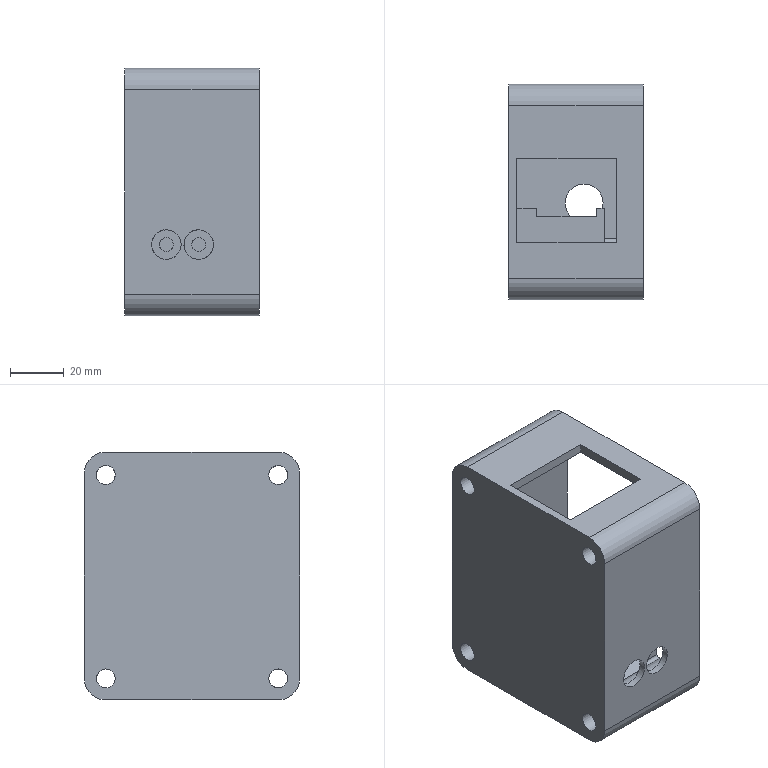NC program | NX | posted by the shop | part box 50 x 80 x 92 mm
Lines 170 to 1000 of 30419:
(T=6 N=D12-36-D12-120-3T-finish D=12.00 R=0.00 FL=45.00 L=120.00)
(XY-STOCK=0.15)
T6 M6
T7
G0 G90 G54 X-66.05 Y-33.361 S6500 M3
G43 H06 Z30.
M8
Z-22.
G1 X-65.9 Y-33.363 Z-22.937 F2000.
X-65.75 Y-33.364 Z-23.308
X-65.6 Y-33.365 Z-23.58
X-65.45 Y-33.367 Z-23.8
X-65.3 Y-33.368 Z-23.984
X-65.15 Y-33.369 Z-24.142
X-65. Y-33.371 Z-24.28
X-64.85 Y-33.372 Z-24.4
X-64.7 Y-33.374 Z-24.505
X-64.55 Y-33.375 Z-24.598
X-64.4 Y-33.376 Z-24.679
X-64.25 Y-33.378 Z-24.75
X-64.1 Y-33.379 Z-24.81
X-63.95 Y-33.38 Z-24.862
X-63.8 Y-33.382 Z-24.905
X-63.65 Y-33.383 Z-24.939
X-63.5 Y-33.384 Z-24.966
X-63.35 Y-33.386 Z-24.985
X-63.2 Y-33.387 Z-24.996
X-63.05 Y-33.388 Z-25.
X-61.193 Y-33.405
G3 X-60.033 Y-32.58 I.011 J1.212
X-59.585 Y-29.553 I-12.064 J3.334
X-59.432 Y-19.77 I-191.621 J7.885
G1 X-59.43 Y-16.803
Y47.501
G2 X-57.211 Y52.214 I6.58 J-.219
X-52.361 Y54.661 I7.101 J-8.045
X-46.379 Y55.335 I6.361 J-29.555
X-33.915 Y55.428 I9.594 J-450.446
G1 X51.556 Y55.427
G2 X56.253 Y53.174 I-.275 J-6.597
X58.654 Y48.401 I-8.065 J-7.048
X59.334 Y42.465 I-29.152 J-6.345
X59.43 Y29.326 I-461.878 J-9.943
G1 X59.428 Y-47.554
G2 X57.143 Y-52.281 I-6.607 J.278
X52.353 Y-54.664 I-7.048 J8.165
X46.506 Y-55.33 I-6.296 J29.24
X33.367 Y-55.428 I-9.91 J449.139
G1 X-51.541 Y-55.427
G2 X-56.242 Y-53.185 I.257 J6.591
X-58.663 Y-48.359 I8.09 J7.078
X-59.333 Y-42.467 I29.289 J6.315
X-59.39 Y-34.774 I126.794 J4.787
G3 X-58.934 Y-27.526 I-175.914 J14.706
X-58.831 Y-14.328 I-499.933 J10.525
G1 X-58.829 Y45.027
G2 X-55.109 Y51.907 I8.591 J-.199
X-49.637 Y54.134 I7.841 J-11.436
X-42.788 Y54.751 I7.155 J-41.068
X-30.144 Y54.828 I10.079 J-620.945
G1 X49.033 Y54.826
G2 X55.893 Y51.133 I-.197 J-8.582
X58.139 Y45.622 I-11.398 J-7.859
X58.754 Y38.728 I-41.439 J-7.174
X58.829 Y25.858 I-648.007 J-10.203
G1 X58.827 Y-45.032
G2 X55.145 Y-51.883 I-8.58 J.196
X49.633 Y-54.134 I-7.864 J11.38
X42.738 Y-54.753 I-7.179 J41.323
X29.869 Y-54.828 I-10.202 J645.306
G1 X-49.033 Y-54.826
G2 X-55.884 Y-51.143 I.197 J8.581
X-58.136 Y-45.633 I11.374 J7.863
X-58.75 Y-38.874 I40.722 J7.109
X-58.549 Y-31.841 I72.756 J1.438
G3 X-58.234 Y-17.292 I-249.929 J12.689
G1 X-58.231 Y-12.843
X-58.23 Y42.657
G2 X-55.478 Y49.812 I9.889 J.304
X-49.82 Y53.049 I8.956 J-9.091
X-43.473 Y54.025 I7.568 J-28.105
X-33.396 Y54.222 I8.68 J-185.849
G1 X-26.961 Y54.227
X46.784 Y54.226
G2 X55.547 Y49.295 I.185 J-9.925
X57.613 Y43.325 I-14.37 J-8.315
X58.167 Y35.836 I-53.023 J-7.684
X58.228 Y24.317 I-720.5 J-9.634
G1 X58.227 Y-42.782
G2 X53.365 Y-51.502 I-9.908 J-.191
X47.54 Y-53.574 I-8.277 J14.05
X40.415 Y-54.151 I-7.539 J48.744
X28.355 Y-54.227 I-10.043 J640.194
G1 X-46.784 Y-54.225
G2 X-55.479 Y-49.404 I-.194 J9.902
X-57.575 Y-43.538 I13.98 J8.304
X-58.04 Y-34.476 I43.348 J6.765
G3 X-57.633 Y-14.776 I-369.169 J17.479
G1 X-57.631 Y40.392
G2 X-57.018 Y45.008 I13.907 J.502
X-51.73 Y51.094 I10.34 J-3.644
X-45.529 Y53.036 I8.624 J-16.67
X-37.633 Y53.568 I8.096 J-61.247
X-25.258 Y53.627 I9.782 J-759.397
G1 X44.668 Y53.626
G2 X49.73 Y52.742 I.396 J-12.668
X55.242 Y47.456 I-4.495 J-10.203
X57.089 Y41.179 I-17.538 J-8.571
X57.584 Y32.829 I-69.072 J-8.283
X57.628 Y20.904 I-783.028 J-8.881
G1 X57.627 Y-40.667
G2 X56.744 Y-45.728 I-12.678 J-.395
X51.405 Y-51.266 I-10.214 J4.506
X45.121 Y-53.095 I-8.561 J17.702
X36.77 Y-53.583 I-8.272 J69.873
X24.89 Y-53.627 I-8.832 J782.468
G1 X-44.668 Y-53.626
G2 X-49.73 Y-52.742 I-.395 J12.678
X-55.267 Y-47.403 I4.505 J10.214
X-57.108 Y-40.985 I17.59 J8.517
X-57.351 Y-33.257 I49.862 J5.435
G3 X-57.032 Y-11.133 I-539.724 J18.847
G1 X-57.031 Y38.727
G2 X-56.496 Y43.45 I16.681 J.504
X-50.884 Y50.302 I11.023 J-3.304
X-44.446 Y52.375 I9.066 J-17.113
X-36.373 Y52.957 I8.421 J-60.577
X-23.999 Y53.026 I10.338 J-741.403
G1 X42.841 Y53.025
G2 X47.689 Y52.421 I.469 J-15.997
X54.309 Y46.873 I-3.551 J-10.961
X56.351 Y40.605 I-16.966 J-8.994
X56.956 Y32.489 I-58.8 J-8.463
X57.028 Y18.63 I-787.178 J-11.01
G1 X57.027 Y-38.822
G2 X56.454 Y-43.585 I-16.194 J-.469
X50.884 Y-50.301 I-10.979 J3.438
X44.563 Y-52.356 I-9.027 J17.015
X36.716 Y-52.949 I-8.324 J57.93
X23.847 Y-53.026 I-10.769 J722.444
G1 X-42.824 Y-53.025
G2 X-47.586 Y-52.453 I-.469 J16.195
X-54.302 Y-46.883 I3.438 J10.98
X-56.377 Y-40.245 I16.639 J8.843
X-56.692 Y-32.699 I49.548 J5.852
G3 X-56.432 Y-10.683 I-719.955 J19.513
G1 X-56.431 Y36.837
G2 X-56.043 Y41.626 I21.951 J.632
X-50.036 Y49.556 I11.703 J-2.625
X-43.439 Y51.721 I9.416 J-17.561
X-35.414 Y52.341 I8.614 J-59.257
X-20.925 Y52.426 I11.55 J-735.565
G1 X41.158 Y52.425
G2 X46.113 Y51.922 I.532 J-19.428
X53.596 Y45.967 I-3.122 J-11.602
X55.706 Y39.542 I-17.567 J-9.327
X56.338 Y31.608 I-57.664 J-8.586
X56.427 Y17.119 I-687.489 J-11.497
G1 Y-36.842
G2 X56.05 Y-41.587 I-22.034 J-.635
X49.974 Y-49.591 I-11.719 J2.589
X43.5 Y-51.71 I-9.349 J17.608
X35.251 Y-52.345 I-8.726 J59.472
X20.897 Y-52.426 I-11.543 J775.238
G1 X-40.843
G2 X-45.588 Y-52.048 I-.633 J22.054
X-53.592 Y-45.968 I2.578 J11.701
X-55.685 Y-39.254 I16.907 J8.953
X-56.036 Y-31.889 I51.489 J6.146
G3 X-55.833 Y-9.199 I-986.222 J20.177
G1 X-55.832 Y34.961
G2 X-55.538 Y39.941 I29.145 J.781
X-48.977 Y48.964 I12.341 J-2.077
X-42.365 Y51.093 I9.596 J-18.477
X-34.387 Y51.729 I8.768 J-59.601
X-19.358 Y51.826 I11.852 J-673.592
G1 X39.268 Y51.825
G2 X44.331 Y51.46 I.694 J-25.69
X52.873 Y45.143 I-2.432 J-12.222
X55.062 Y38.557 I-17.984 J-9.634
X55.726 Y30.536 I-57.633 J-8.813
X55.827 Y15.057 I-663.748 J-12.064
G1 Y-35.312
G2 X55.453 Y-40.374 I-25.27 J-.682
X49.038 Y-48.929 I-12.234 J2.491
X42.347 Y-51.095 I-9.65 J18.397
X33.873 Y-51.742 I-9.002 J62.053
X19.024 Y-51.826 I-11.863 J788.145
G1 X-39.313 Y-51.825
G2 X-44.376 Y-51.452 I-.682 J25.271
X-52.969 Y-44.944 I2.473 J12.194
X-55.022 Y-38.126 I17.756 J9.063
X-55.384 Y-30.265 I57.878 J6.605
G1 X-55.26 Y-19.515
X-55.233 Y-9.153
X-55.232 Y33.237
G2 X-54.977 Y38.536 I36.153 J.914
X-48.019 Y48.341 I12.855 J-1.75
X-41.178 Y50.494 I9.863 J-19.401
X-32.523 Y51.14 I9.224 J-65.201
X-17.673 Y51.225 I11.964 J-795.405
G1 X37.963 Y51.224
G2 X43.252 Y50.849 I.682 J-27.83
X52.246 Y44.194 I-2.418 J-12.674
X54.455 Y37.42 I-18.845 J-9.892
X55.137 Y28.723 I-62.607 J-9.285
X55.227 Y13.379 I-763.643 J-12.131
G1 X55.226 Y-33.962
G2 X54.85 Y-39.25 I-27.809 J-.682
X48.092 Y-48.3 I-12.7 J2.436
X41.165 Y-50.495 I-9.925 J19.292
X32.735 Y-51.135 I-9.114 J64.191
X17.391 Y-51.225 I-12.16 J764.582
G1 X-37.558
G2 X-42.809 Y-50.929 I-.816 J32.224
X-52.394 Y-43.858 I1.974 J12.708
X-54.374 Y-36.967 I18.877 J9.154
X-54.744 Y-28.611 I65.348 J7.079
G1 X-54.661 Y-19.337
X-54.633 Y-7.489
X-54.632 Y31.961
G2 X-54.367 Y37.485 I38.814 J.903
X-47.153 Y47.69 I13.26 J-1.722
X-40.185 Y49.872 I10.075 J-19.948
X-31.397 Y50.535 I9.43 J-66.433
X-16.052 Y50.625 I12.267 J-787.77
G1 X36.118 Y50.624
G2 X41.64 Y50.338 I.874 J-36.553
X51.695 Y43.143 I-1.864 J-13.227
X53.876 Y36.172 I-19.983 J-10.077
X54.531 Y27.563 I-65.673 J-9.328
X54.626 Y11.904 I-745.433 J-12.373
G1 Y-32.297
G2 X54.311 Y-37.817 I-34.27 J-.812
X47.178 Y-47.674 I-13.19 J2.035
X40.249 Y-49.861 I-10.075 J19.849
X31.686 Y-50.528 I-9.339 J64.607
X16.207 Y-50.625 I-12.277 J724.209
G1 X-36.298 Y-50.624
G2 X-41.818 Y-50.309 I-.812 J34.267
X-51.727 Y-42.979 I1.983 J13.043
X-53.712 Y-35.997 I19.559 J9.336
X-54.111 Y-27.552 I67.427 J7.418
G1 X-54.106 Y28.127
G2 X-53.946 Y34.695 I202.242 J-1.656
X-52.371 Y41.027 I16.21 J-.67
X-45.82 Y47.292 I12.448 J-6.458
X-38.708 Y49.333 I10.142 J-21.928
X-29.734 Y49.944 I9.569 J-74.278
X-14.884 Y50.024 I11.838 J-816.458
G1 X34.858
G2 X40.561 Y49.739 I.88 J-39.624
X51.063 Y42.273 I-1.773 J-13.612
X53.235 Y35.338 I-20.43 J-10.209
X53.915 Y26.821 I-64.515 J-9.438
X54.026 Y9.992 I-718.885 J-13.131
G1 X54.024 Y-31.127
G2 X53.719 Y-36.693 I-37.081 J-.757
X46.284 Y-47.054 I-13.582 J1.898
X39.133 Y-49.267 I-10.304 J20.643
X30.209 Y-49.933 I-9.611 J68.627
X15.809 Y-50.024 I-11.908 J744.31
G1 X-34.948
G2 X-40.694 Y-49.718 I-.861 J37.983
X-51.099 Y-42.046 I1.844 J13.393
X-53.057 Y-35.055 I20.323 J9.46
X-53.482 Y-27.241 I66.6 J7.544
G1 X-53.511 Y-16.441
Y27.959
G2 X-53.289 Y34.401 I94.275 J-.023
X-51.236 Y41.105 I15.589 J-1.108
X-44.581 Y46.843 I12.443 J-7.703
X-37.212 Y48.794 I10.282 J-23.952
X-27.829 Y49.358 I9.816 J-84.995
X-13.474 Y49.424 I11.025 J-831.87
G1 X33.553 Y49.423
G2 X39.482 Y49.145 I.923 J-43.625
X47.738 Y45.164 I-1.672 J-14.018
X51.696 Y38.346 I-12.088 J-11.576
X53.07 Y30.563 I-33.2 J-9.873
X53.405 Y19.321 I-163.826 J-10.512
G1 X53.425 Y8.341
X53.423 Y-29.744
G2 X53.123 Y-35.626 I-41.476 J-.831
X45.462 Y-46.411 I-13.931 J1.782
X38.445 Y-48.61 I-10.395 J20.877
X29.345 Y-49.324 I-9.845 J67.114
X14.495 Y-49.424 I-12.125 J699.19
G1 X-33.778 Y-49.423
G2 X-39.571 Y-49.131 I-.829 J41.203
X-47.636 Y-45.219 I1.715 J13.808
X-51.513 Y-38.427 I11.639 J11.146
X-52.705 Y-30.933 I31.673 J8.876
X-52.903 Y-21.081 I187.566 J8.699
G1 X-52.911 Y-13.431
Y27.954
G2 X-52.623 Y34.065 I61.365 J.173
X-50.029 Y41.189 I15.224 J-1.509
X-43.255 Y46.428 I12.408 J-9.042
X-35.844 Y48.236 I10.299 J-26.12
X-25.917 Y48.769 I10.152 J-96.446
X-12.058 Y48.824 I10.255 J-846.354
G1 X32.417 Y48.822
G2 X38.437 Y48.55 I.906 J-46.549
X46.197 Y45.236 I-1.646 J-14.598
X50.743 Y38.448 I-10.66 J-12.056
X51.739 Y35.385 I-123.155 J-41.738
X52.554 Y28.424 I-46.333 J-8.955
X52.815 Y15.739 I-246.366 J-11.4
G1 X52.825 Y6.919
X52.822 Y-28.871
G2 X52.496 Y-34.797 I-41.001 J-.719
X48.173 Y-43.306 I-14.226 J1.874
X41.273 Y-47.136 I-11.657 J12.873
X33.301 Y-48.482 I-10.077 J35.382
X21.473 Y-48.809 I-10.779 J176.117
G1 X12.068 Y-48.823
X-32.518 Y-48.822
G2 X-38.626 Y-48.522 I-.894 J44.051
X-46.362 Y-45.043 I1.746 J14.224
X-50.545 Y-38.542 I10.675 J11.464
G1 X-51.231 Y-37.017
X-51.739 Y-35.385
X-52.047 Y-33.705
G2 X-52.15 Y-30.11 I32.143 J2.721
X-52.31 Y-13.553 I526.769 J13.358
G1 Y27.94
G2 X-52.047 Y33.706 I131.583 J-3.127
X-51.553 Y36.036 I17.054 J-2.399
X-43.691 Y45.235 I14.29 J-4.253
X-36.259 Y47.443 I10.765 J-22.622
X-26.75 Y48.129 I10.209 J-75.315
X-10.191 Y48.223 I13.13 J-853.131
G1 X34.014
G2 X39.828 Y47.492 I-.321 J-26.043
X47.386 Y42.589 I-3.537 J-13.727
G1 X48.592 Y41.382
X49.646 Y40.037
X50.53 Y38.575
X51.231 Y37.017
X51.739 Y35.385
X52.047 Y33.705
X52.15 Y32.
Y-32.
X52.047 Y-33.706
X51.739 Y-35.387
G2 X50.414 Y-38.821 I-16.55 J4.411
X43.173 Y-45.48 I-13.39 J7.294
X35.727 Y-47.52 I-10.627 J24.184
X26.033 Y-48.144 I-10.224 J83.158
X10.284 Y-48.223 I-12.175 J860.387
G1 X-34.378 Y-48.208
G2 X-40.199 Y-47.382 I.41 J23.815
X-47.133 Y-42.791 I3.866 J13.369
X-48.592 Y-41.382 I11.358 J13.225
G1 X-49.646 Y-40.037
X-50.548 Y-38.534
X-49.646 Y-40.037
X-48.592 Y-41.382
G3 X-47.167 Y-42.761 I12.469 J11.467
X-43.341 Y-45.467 I18.584 J22.216
X-36.097 Y-47.62 I8.837 J16.468
X-29.759 Y-47.851 I5.681 J68.79
G1 X-22.649 Y-47.863
X34.576
G2 X35.147 Y-48.007 I-.004 J-1.218
G1 X35.889 Y-48.504 Z-24.962
X36.623 Y-49.014 Z-24.925
X37.11 Y-49.35 Z-24.9
X38.531 Y-50.327 F10000.
G3 X39.212 Y-50.539 I.683 J.997
G1 X40.25 Y-50.53
G3 X41.406 Y-50.312 I-.308 J4.819
G1 X42.378 Y-50.003
X43.345 Y-49.679
G3 X46.735 Y-47.846 I-4.616 J12.589
G1 X49.967 Y-45.439
G3 X51.86 Y-43.39 I-4.537 J6.091
G1 X52.615 Y-42.188
G3 X52.78 Y-41.762 I-1.078 J.662
G1 X53.076 Y-40.118
X53.496 Y-37.776 Z-25. F2000.
G3 X51.23 Y-37.018 I-1.171 J.264
G1 X50.529 Y-38.577
X49.645 Y-40.039
X48.591 Y-41.384
X47.382 Y-42.592
X46.037 Y-43.646
X44.575 Y-44.53
X43.017 Y-45.231
G2 X38.385 Y-46.396 I-10.226 J30.855
X30.203 Y-47.206 I-8.318 J42.298
X17.963 Y-47.262 I-9.605 J760.85
G1 X-34.042 Y-47.26
G2 X-40.299 Y-45.938 I2.421 J26.922
G1 X-41.387 Y-45.739
X-43.018 Y-45.23
X-44.577 Y-44.529
X-46.039 Y-43.645
X-44.577 Y-44.529
X-43.018 Y-45.23
X-41.387 Y-45.739
G3 X-35.32 Y-46.686 I17.608 J92.85
X-28.71 Y-46.893 I5.815 J80.113
G1 X-22.95 Y-46.902
X34.59 Y-46.9
G2 X37.857 Y-46.158 I65.751 J-282.065
G1 X39.705 Y-46.047
X41.385 Y-45.739
X39.705 Y-46.047
G2 X36.912 Y-46.15 I-2.393 J26.934
X26.246 Y-46.299 I-8.557 J230.339
G1 X-33.994 Y-46.301
X-35.108 Y-46.15
G2 X-39.706 Y-46.047 I-1.203 J48.841
G1 X-38. Y-46.15
X36.937
G2 X37.778 Y-48.206 I0.0 J-1.2
X37.24 Y-48.517 Z-24.974 I-.924 J.979
G1 X35.595 Y-49.119 Z-24.9
X33.565 Y-49.862 F10000.
X33.362 Y-49.915
X33.152 Y-49.935
X-37.468
G2 X-42.948 Y-49.177 I-.046 J19.873
X-46.005 Y-47.896 I4.401 J14.79
X-48.323 Y-46.497 I11.078 J20.974
X-51.573 Y-43.612 I11.236 J15.934
X-54.813 Y-37.858 I10.293 J9.584
G1 X-55.935 Y-33.894
G2 X-55.337 Y-32.504 I1.155 J.327
G1 X-55.127 Y-32.395
X-53.02 Y-31.291 Z-25. F2000.
G3 X-52.528 Y-30.984 I-.836 J1.885
X-52.15 Y-30.11 I-.824 J.875
G1 Y32.
X-52.047 Y33.706
X-51.739 Y35.387
X-51.23 Y37.018
X-50.529 Y38.577
X-49.645 Y40.039
X-48.591 Y41.384
X-47.382 Y42.592
X-46.037 Y43.646
X-44.575 Y44.53
X-43.017 Y45.231
G2 X-38.169 Y46.439 I10.515 J-31.858
X-27.701 Y47.471 I11.867 J-66.781
X-12.582 Y47.621 I12.624 J-509.133
G1 X34.008 Y47.623
G2 X40.034 Y46.573 I-.881 J-22.88
X42.9 Y45.267 I-6.828 J-18.784
G1 X44.577 Y44.529
X46.039 Y43.645
X47.416 Y42.559
X46.039 Y43.645
X44.577 Y44.529
X42.9 Y45.267
G3 X38.703 Y46.511 I-18.892 J-56.034
X32.229 Y47.213 I-6.507 J-29.788
X22.239 Y47.262 I-8.328 J-682.107
G1 X-33.991
G2 X-34.561 Y47.407 I.004 J1.218
X-35.163 Y48.184 Z-24.958 I.618 J1.101
G1 X-35.604 Y49.479 Z-24.9
X-35.938 Y50.46 F10000.
G3 X-37.775 Y51.047 I-1.136 J-.387
G1 X-38.729 Y50.36
X-40.909 Y48.855
X-42.339 Y47.863 Z-24.973 F2000.
G3 X-42.718 Y47.36 Z-25. I.742 J-.952
X-41.385 Y45.739 I1.116 J-.44
G1 X-39.705 Y46.047
G3 X-33.372 Y46.502 I-15.361 J257.906
G2 X-23.835 Y46.658 I7.936 J-193.701
G1 X-18.075 Y46.662
X34.05 Y46.66
G2 X37.203 Y46.15 I-24.159 J-159.377
X39.706 Y46.047 I.174 J-26.162
G1 X41.387 Y45.739
X42.032 Y45.538
X41.387 Y45.739
X39.706 Y46.047
G3 X36.26 Y46.161 I-3.049 J-40.01
X28.03 Y46.299 I-6.731 J-155.436
G1 X23.98 Y46.301
X-31.875 Y46.3
X-33.546 Y46.15
X-38.
X36.609
G3 X37.82 Y47.402 I0.0 J1.212
G1 X37.764 Y49.123
X37.759 Y49.273 Z-24.996
X37.754 Y49.423 Z-24.985
X37.749 Y49.573 Z-24.966
X37.744 Y49.723 Z-24.939
X37.739 Y49.873 Z-24.905
X37.734 Y50.023 Z-24.862
X37.729 Y50.173 Z-24.81
X37.725 Y50.323 Z-24.75
X37.72 Y50.473 Z-24.679
X37.715 Y50.623 Z-24.598
X37.71 Y50.773 Z-24.505
X37.705 Y50.922 Z-24.4
X37.7 Y51.072 Z-24.28
X37.695 Y51.222 Z-24.142
X37.69 Y51.372 Z-23.984
X37.685 Y51.522 Z-23.8
X37.68 Y51.672 Z-23.58
X37.675 Y51.822 Z-23.308
X37.67 Y51.972 Z-22.937
X37.666 Y52.122 Z-22.
G0 Z30.
X-21.441 Y-5.314
Z3.
G3 X-21.441 Y-5.314 Z2.408 I.959 J5.314
X-21.441 Y-5.314 Z1.816 I.959 J5.314
X-21.441 Y-5.314 Z1.223 I.959 J5.314
X-21.441 Y-5.314 Z.631 I.959 J5.314
X-21.441 Y-5.314 Z.039 I.959 J5.314
X-21.441 Y-5.314 Z-.553 I.959 J5.314
X-21.441 Y-5.314 Z-1.146 I.959 J5.314
X-21.441 Y-5.314 Z-1.738 I.959 J5.314
X-21.441 Y-5.314 Z-2.33 I.959 J5.314
X-21.441 Y-5.314 Z-2.922 I.959 J5.314
X-21.441 Y-5.314 Z-3.515 I.959 J5.314
X-21.441 Y-5.314 Z-4.107 I.959 J5.314
X-21.441 Y-5.314 Z-4.699 I.959 J5.314
X-21.441 Y-5.314 Z-5.291 I.959 J5.314
X-21.441 Y-5.314 Z-5.884 I.959 J5.314
X-21.441 Y-5.314 Z-6.476 I.959 J5.314
X-21.441 Y-5.314 Z-7.068 I.959 J5.314
X-21.441 Y-5.314 Z-7.66 I.959 J5.314
X-21.441 Y-5.314 Z-8.252 I.959 J5.314
X-21.441 Y-5.314 Z-8.845 I.959 J5.314
X-21.441 Y-5.314 Z-9.437 I.959 J5.314
X-21.441 Y-5.314 Z-10.029 I.959 J5.314
X-21.441 Y-5.314 Z-10.621 I.959 J5.314
X-21.441 Y-5.314 Z-11.214 I.959 J5.314
X-21.441 Y-5.314 Z-11.806 I.959 J5.314
X-21.441 Y-5.314 Z-12.398 I.959 J5.314
X-21.441 Y-5.314 Z-12.99 I.959 J5.314
X-21.441 Y-5.314 Z-13.583 I.959 J5.314
X-21.441 Y-5.314 Z-14.175 I.959 J5.314
X-21.441 Y-5.314 Z-14.767 I.959 J5.314
X-21.441 Y-5.314 Z-15.359 I.959 J5.314
X-21.441 Y-5.314 Z-15.952 I.959 J5.314
X-21.441 Y-5.314 Z-16.544 I.959 J5.314
X-21.441 Y-5.314 Z-17.136 I.959 J5.314
X-21.441 Y-5.314 Z-17.728 I.959 J5.314
X-21.441 Y-5.314 Z-18.321 I.959 J5.314
X-21.441 Y-5.314 Z-18.913 I.959 J5.314
X-21.441 Y-5.314 Z-19.505 I.959 J5.314
X-21.441 Y-5.314 Z-20.097 I.959 J5.314
X-21.441 Y-5.314 Z-20.689 I.959 J5.314
X-21.441 Y-5.314 Z-21.282 I.959 J5.314
X-21.441 Y-5.314 Z-21.874 I.959 J5.314
X-21.441 Y-5.314 Z-22.466 I.959 J5.314
X-21.441 Y-5.314 Z-23.058 I.959 J5.314
X-21.441 Y-5.314 Z-23.651 I.959 J5.314
X-21.441 Y-5.314 Z-24.243 I.959 J5.314
X-21.441 Y-5.314 Z-24.835 I.959 J5.314
X-15.081 Y0.0 Z-25. I.959 J5.314
X-22.765 Y-4.95 I-5.425 J-.017
X-15.264 Y-1.703 I2.29 J4.997
X-21.571 Y5.586 I-5.203 J1.871
X-15.533 Y-2.918 I1.11 J-5.607
X-22.691 Y5.546 I-4.958 J3.065
X-15.421 Y-3.273 I2.235 J-5.563
X-23.24 Y5.612 I-5.08 J3.413
X-15.368 Y-3.7 I2.784 J-5.63
X-23.479 Y5.818 I-5.137 J3.837
X-15.383 Y-4.196 I3.024 J-5.835
X-23.901 Y5.927 I-5.128 J4.33
X-15.482 Y-4.757 I3.446 J-5.943
X-24.742 Y5.736 I-5.037 J4.887
X-15.464 Y-5.172 I4.288 J-5.752
X-24.549 Y6.248 I-5.055 J5.303
X-15.755 Y-5.842 I4.093 J-6.266
X-24.774 Y6.479 I-4.766 J5.973
X-15.673 Y-6.185 I4.321 J-6.497
X-24.928 Y6.762 I-4.849 J6.316
X-15.667 Y-6.585 I4.475 J-6.782
X-25.008 Y7.098 I-4.853 J6.718
X-15.743 Y-7.04 I4.554 J-7.121
X-25.014 Y7.489 I-4.779 J7.173
X-15.632 Y-7.371 I4.56 J-7.513
X-24.934 Y7.928 I-4.89 J7.505
X-15.596 Y-7.754 I4.482 J-7.952
X-24.766 Y8.408 I-4.924 J7.888
X-15.932 Y-8.352 I4.314 J-8.434
X-24.504 Y8.922 I-4.589 J8.487
X-16.38 Y-8.968 I4.05 J-8.95
X-23.146 Y9.779 I-4.132 J9.103
X-19.325 Y-10.138 I2.677 J-9.812
X-22.294 Y10.334 I-1.177 J10.28
X-20.8 Y-10.557 I1.819 J-10.369
X-20.958 Y10.838 I.306 J10.701
X-22.749 Y-10.683 I.469 J-10.874
X-16.987 Y10.637 I2.278 J10.823
X-26.078 Y-9.793 I-3.528 J-10.668
X-11.028 Y6.561 I5.646 J9.906
X-32.087 Y-.829 I-9.532 J-6.537
X-9.846 Y-5.027 I11.68 J.866
X-27.488 Y9.737 I-10.699 J5.138
X-13.255 Y-9.7 I7.05 J-9.767
X-23.964 Y11.864 I-7.262 J9.835
X-21.181 Y-12.426 I3.496 J-11.904
X-17.945 Y12.47 I.695 J12.568
X-28.178 Y-10.237 I-2.562 J-12.504
X-8.535 Y5.173 I7.757 J10.336
X-33.482 Y2.125 I-12.033 J-5.133
X-8.81 Y-6.401 I13.081 J-2.107
X-29.271 Y10.317 I-11.743 J6.508
X-12.826 Y-11.319 I8.841 J-10.348
X-25.159 Y13.131 I-7.702 J11.45
X-17.44 Y-13.706 I4.701 J-13.176
X-18.226 Y14.131 I-3.055 J13.844
X-31.493 Y-9.266 I-2.288 J-14.162
X-5.964 Y1.348 I11.089 J9.337
X-34.896 Y3.234 I-14.612 J-1.292
X-8.961 Y-9.462 I14.494 J-3.23
X-30.647 Y11.26 I-11.592 J9.577
X-11.872 Y-12.641 I10.229 J-11.289
X-21.701 Y15.51 I-8.654 J12.77
X-25.773 Y-14.729 I1.221 J-15.559
X-6.087 Y6.632 I5.34 J14.831
X-18.54 Y15.85 I-14.427 J-6.47
X-22.34 Y15.82 I-1.34 J-70.753
X-33.885 Y8.772 I1.536 J-15.495
X-36.35 Y2.207 I13.315 J-8.746
X-36.321 Y-1.936 I80.621 J-1.502
X-29.721 Y-13.151 I15.498 J1.571
X-23.222 Y-15.85 I9.209 J13.
X-18.219 Y-15.829 I1.797 J171.551
X-9.938 Y-12.238 I-1.513 J14.832
X-16.282 Y15.839 I-10.579 J12.365
G1 X-18.554 Y15.85
X-16.04 Y15.835
G2 X-12.176 Y14.392 I-1.793 J-10.695
X-13.822 Y-14.956 I-8.29 J-14.255
X-16.726 Y-15.85 I-5.185 J11.679
G1 X-18.616
G3 X-15.839 Y-15.831 I.778 J89.508
X-11.528 Y-14.224 I-1.614 J10.92
X-5.401 Y7.843 I-8.866 J14.345
X-13.633 Y15.58 I-14.62 J-7.308
X-14.537 Y15.85 I-1.403 J-3.043
G1 X-16.247
X-14.236 Y15.833
G2 X-11.029 Y14.475 I-1.825 J-8.773
X-4.282 Y-5.676 I-9.381 J-14.346
X-12.76 Y-15.16 I-15.635 J5.444
X-14.821 Y-15.85 I-3.539 J7.151
G1 X-16.126
G3 X-14.097 Y-15.823 I.725 J21.74
X-10.434 Y-14.299 I-1.739 J9.347
X-2.902 Y-1.416 I-9.581 J14.243
X-10.466 Y14.624 I-17.423 J1.588
X-12.914 Y15.835 I-5.044 J-7.116
G1 X-14.443 Y15.85
G2 X-12.747 Y15.829 I.597 J-20.608
X-9.895 Y14.505 I-1.852 J-7.72
X-2.895 Y3.504 I-10.072 J-14.136
X-9.316 Y-13.822 I-17.338 J-3.428
X-13.201 Y-15.834 I-6.981 J8.725
G1 X-14.416 Y-15.85
G3 X-12.572 Y-15.799 I.596 J11.864
X-9.074 Y-14.127 I-2.091 J8.869
X-2.557 Y-3.864 I-10.49 J13.862
X-8.43 Y13.937 I-17.764 J4.008
X-11.531 Y15.817 I-6.795 J-7.711
X-12.924 Y15.85 I-.915 J-9.222
G2 X-11.446 Y15.825 I.554 J-10.999
X-8.744 Y14.468 I-1.889 J-7.128
X-2.82 Y6.048 I-10.619 J-13.765
X-7.049 Y-12.723 I-17.456 J-5.929
X-11.414 Y-15.68 I-8.949 J8.511
X-12.076 Y-15.85 I-1.174 J3.195
G1 X-12.976
G3 X-11.362 Y-15.799 I.499 J9.894
X-8.139 Y-14.205 I-1.994 J8.083
X-2.505 Y-6.285 I-10.596 J13.502
X-6.672 Y13.242 I-17.8 J6.41
X-10.235 Y15.779 I-8.098 J-7.601
G1 X-10.587 Y15.85
X-11.667
G2 X-10.286 Y15.826 I.501 J-10.764
X-7.76 Y14.51 I-1.799 J-6.537
X-2.61 Y7.552 I-10.717 J-13.317
X-5.4 Y-11.929 I-17.645 J-7.414
X-9.744 Y-15.458 I-10.258 J8.189
X-10.917 Y-15.85 I-1.844 J3.572
G1 X-11.772
G3 X-10.24 Y-15.798 I.488 J8.259
X-7.157 Y-14.215 I-1.945 J7.581
X-2.058 Y-7.15 I-10.758 J13.136
X-5.213 Y12.68 I-18.179 J7.274
X-8.834 Y15.644 I-9.139 J-7.47
X-9.508 Y15.85 I-.868 J-1.633
G1 X-10.498
G2 X-9.201 Y15.825 I.462 J-9.833
X-6.726 Y14.482 I-1.761 J-6.194
X-2.064 Y8.128 I-10.904 J-12.889
X-3.982 Y-11.234 I-18.13 J-7.979
X-8.346 Y-15.281 I-11.221 J7.722
X-9.839 Y-15.85 I-2.299 J3.794
G1 X-10.649
G3 X-9.17 Y-15.795 I.444 J7.947
X-6.15 Y-14.175 I-1.979 J7.318
X-1.389 Y-7.433 I-11.013 J12.828
X-3.877 Y12.138 I-18.751 J7.56
X-7.543 Y15.507 I-10.027 J-7.232
X-8.464 Y15.85 I-1.25 J-1.95
G1 X-9.454
G2 X-8.159 Y15.823 I.475 J-8.373
X-5.746 Y14.468 I-1.76 J-5.957
X-1.41 Y8.46 I-11.003 J-12.51
X-2.861 Y-10.842 I-18.663 J-8.303
X-6.968 Y-15.054 I-11.895 J7.49
X-8.782 Y-15.847 I-2.946 J4.27
G1 X-9.592 Y-15.85
G3 X-8.157 Y-15.793 I.448 J6.792
X-5.969 Y-14.664 I-.992 J4.61
X-2.469 Y-11.029 I-7.158 J10.392
X.544 Y3.463 I-17.205 J11.136
X-3.919 Y13.278 I-19.338 J-2.871
X-4.636 Y13.838 I-1.347 J-.986
G1 X-5.856 Y14.582
G3 X-7.261 Y15.692 I-6.938 J-7.334
X-8.401 Y15.85 I-.883 J-2.18
G2 X-7.339 Y15.738 I.245 J-2.761
X-6.821 Y15.4 I-1.916 J-3.502
G3 X-4.514 Y13.788 I6.51 J6.861
G2 X-3.436 Y12.944 I-1.437 J-2.946
X-.26 Y7.586 I-12.055 J-10.766
X-1.714 Y-10.332 I-19.643 J-7.424
X-4.42 Y-13.732 I-12.742 J7.363
G3 X-5.756 Y-14.528 I5.392 J-10.577
G2 X-4.207 Y-13.648 I4.838 J-6.711
G3 X-1.896 Y-11.334 I-4.698 J7.004
X1.415 Y-2.31 I-15.967 J10.976
X-1.423 Y11.012 I-20.88 J2.515
X-3.193 Y13.213 I-8.279 J-4.844
X-4.464 Y13.767 I-5.008 J-9.745
G2 X-3.084 Y13.17 I-4.111 J-11.389
X-1.092 Y10.902 I-4.84 J-6.259
X1.808 Y1.186 I-17.298 J-10.454
X-.965 Y-10.393 I-20.679 J-1.17
X-3.385 Y-13.288 I-9.142 J5.184
G1 X-3.627 Y-13.407
G2 X-4.656 Y-13.243 I-.344 J1.151
G1 X-4.909 Y-13.067
X-6.861 Y-11.709 Z-24.9
X-8.262 Y-10.731 F10000.
X-8.473 Y-10.563
X-8.692 Y-10.404
G3 X-10.472 Y-11.709 I-.611 J-1.033
G1 X-10.204 Y-12.861
X-9.707 Y-14.984 Z-24.992 F2000.
X-9.638 Y-15.169 Z-25.
G3 X-8.557 Y-15.85 I1.082 J.52
X-7.079 Y-15.593 I.284 J2.753
G1 X-6.339 Y-14.983
G2 X-7.339 Y-15.738 I-3.327 J3.369
X-8.084 Y-15.85 I-.681 J1.999
G3 X-7.339 Y-15.738 I.103 J1.848
G1 X-6.885 Y-15.453
G2 X-3.294 Y-13.293 I6.519 J-6.77
G3 X-1.25 Y-11.449 I-3.173 J5.575
X1.342 Y-6.206 I-12.395 J9.389
G1 X1.469 Y-4.799
G3 X2.241 Y1.667 I-15.524 J5.134
X-.585 Y10.917 I-19.975 J-1.047
X-2.371 Y13.004 I-6.706 J-3.931
X-3.315 Y13.294 I-1.465 J-3.085
G2 X-2.351 Y13.025 I-.642 J-4.158
X-.496 Y11.152 I-3.313 J-5.137
X2.193 Y4.305 I-15.136 J-9.897
X2.257 Y-2.784 I-18.555 J-3.713
G1 X1.806 Y-3.688
G3 X2.51 Y-2.256 I-11.156 J6.373
X2.931 Y1.899 I-11.305 J3.244
X.311 Y10.695 I-18.862 J-.83
X-1.547 Y12.82 I-6.259 J-3.599
G1 X-1.88 Y12.955
G3 X-2.968 Y12.554 I-.181 J-1.187
X-3.258 Y12.019 Z-24.974 I1.465 J-1.141
G1 X-3.946 Y10.392 Z-24.9
X-4.344 Y9.452 F10000.
G3 X-3.265 Y7.785 I1.105 J-.467
G1 X-2.85 Y7.773
X-2.434 Y7.777
G3 X-1.907 Y9.97 I-.136 J1.192
G1 X-3.549 Y10.964 Z-24.981 F2000.
G2 X-3.872 Y11.286 Z-25. I.692 J1.017
X-2.596 Y13.122 I.996 J.669
X-1.582 Y12.871 I-1.93 J-9.957
X.203 Y11.204 I-2.654 J-4.631
X2.736 Y5.289 I-13.365 J-9.223
X3.059 Y-.917 I-16.252 J-3.958
X2.673 Y-2.227 I-3.738 J.389
G1 X2.345 Y-2.661
X2.861 Y-1.982
G3 X3.555 Y.739 I-5.86 J2.945
X1.045 Y10.704 I-17.179 J.97
X-.906 Y12.777 I-5.644 J-3.356
X-1.926 Y12.962 I-.953 J-2.352
G2 X-.986 Y12.846 I.033 J-3.618
X.797 Y11.366 I-2.031 J-4.259
X3.249 Y6.191 I-11.382 J-8.562
X3.721 Y.099 I-14.795 J-4.21
X3.217 Y-1.571 I-4.5 J.448
G1 X3.162 Y-1.643
G2 X1.515 Y-1.519 I-.758 J.93
X1.235 Y-.419 Z-24.95 I.933 J.823
G1 X1.42 Y.765 Z-24.9
X1.468 Y1.059 F10000.
X1.501 Y1.355
G3 X-.623 Y2.142 I-1.2 J.022
G1 X-.866 Y1.852
X-1.096 Y1.552
G3 X-.986 Y.143 I1.022 J-.629
G1 X-.094 Y-.898
X1.002 Y-2.171 Z-24.971 F2000.
G3 X1.602 Y-2.507 Z-25. I.864 J.838
X2.786 Y-2.096 I.256 J1.173
X3.442 Y-1.311 I-11.727 J10.458
X4.178 Y1.447 I-5.632 J2.979
X1.681 Y10.837 I-15.587 J.882
X-.279 Y12.763 I-5.034 J-3.164